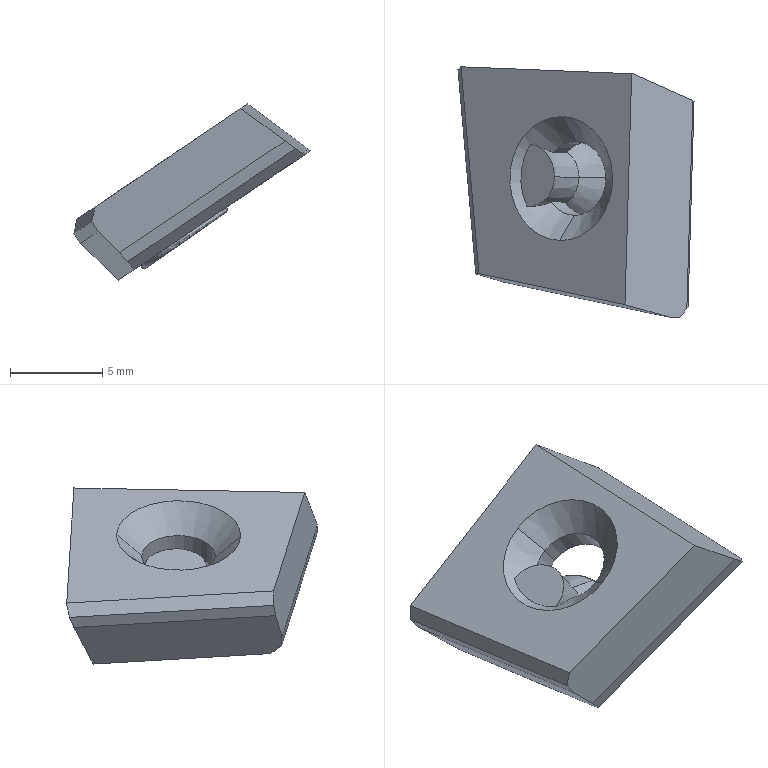Part | SolidWorks | features BaseBody 1 | 1 solid | 29 faces | box 12.787 x 13.574 x 9.538 mm | volume 465.573 mm3 | plane 14 | cone 8 | cylinder 3 | torus 2 | spline 2 | commonest cylinder face diameters 4 x3